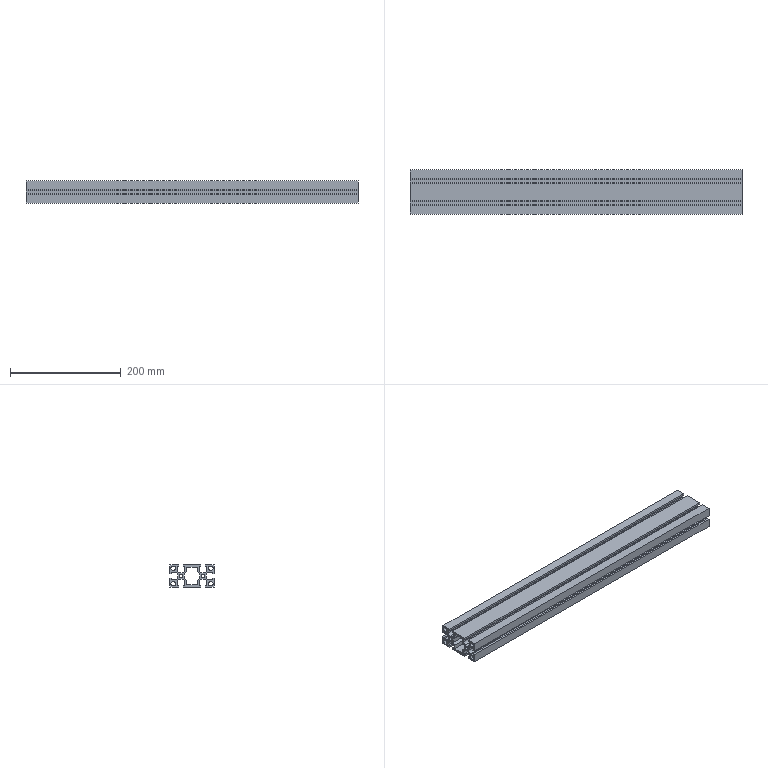Part | SolidWorks | features BaseBody 1 | 1 solid | 90 faces | box 600 x 80 x 40 mm | volume 739462 mm3 | plane 66 | cylinder 24 | commonest cylinder face diameters 10 x12 8 x8 6.2 x4